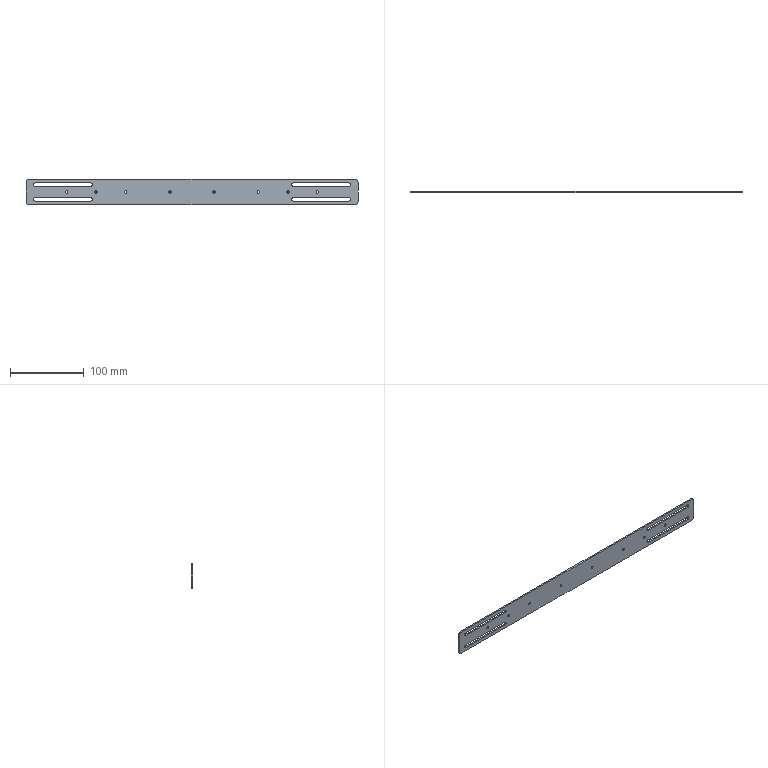Part | SolidWorks | features HoleWzd 3, Fillet 2, Cut 1, EdgeFlange 1, FlatPattern 1, SMBaseFlange 1, SheetMetal 1 | 1 solid | 42 faces | box 450 x 2 x 35 mm | volume 28475 mm3 | cylinder 28 | plane 14 | commonest cylinder face diameters 3.3 x16 4.5 x8 10 x4
STEP:
#1=CARTESIAN_POINT('',(-30.,-2.,-1.65));
#2=VERTEX_POINT('',#1);
#3=CARTESIAN_POINT('',(-30.,-2.,1.65));
#4=VERTEX_POINT('',#3);
#5=CARTESIAN_POINT('',(-30.,-2.,0.));
#6=DIRECTION('',(0.,1.,0.));
#7=DIRECTION('',(0.,0.,1.));
#8=AXIS2_PLACEMENT_3D('',#5,#6,#7);
#9=CIRCLE('',#8,1.65);
#10=EDGE_CURVE('',#2,#4,#9,.T.);
#11=ORIENTED_EDGE('',*,*,#10,.F.);
#12=CARTESIAN_POINT('',(-30.,0.,-1.65));
#13=VERTEX_POINT('',#12);
#14=CARTESIAN_POINT('',(-30.,0.,-1.65));
#15=DIRECTION('',(0.,1.,0.));
#16=VECTOR('',#15,1000.);
#17=LINE('',#14,#16);
#18=EDGE_CURVE('',#2,#13,#17,.T.);
#19=ORIENTED_EDGE('',*,*,#18,.T.);
#20=CARTESIAN_POINT('',(-30.,0.,1.65));
#21=VERTEX_POINT('',#20);
#22=CARTESIAN_POINT('',(-30.,0.,0.));
#23=DIRECTION('',(0.,1.,0.));
#24=DIRECTION('',(0.,0.,1.));
#25=AXIS2_PLACEMENT_3D('',#22,#23,#24);
#26=CIRCLE('',#25,1.65);
#27=EDGE_CURVE('',#13,#21,#26,.T.);
#28=ORIENTED_EDGE('',*,*,#27,.T.);
#29=CARTESIAN_POINT('',(-30.,0.,1.65));
#30=DIRECTION('',(0.,1.,0.));
#31=VECTOR('',#30,1000.);
#32=LINE('',#29,#31);
#33=EDGE_CURVE('',#4,#21,#32,.T.);
#34=ORIENTED_EDGE('',*,*,#33,.F.);
#35=EDGE_LOOP('',(#11,#19,#28,#34));
#36=FACE_OUTER_BOUND('',#35,.T.);
#37=CARTESIAN_POINT('',(-30.,0.,0.));
#38=DIRECTION('',(0.,1.,0.));
#39=DIRECTION('',(0.,0.,1.));
#40=AXIS2_PLACEMENT_3D('',#37,#38,#39);
#41=CYLINDRICAL_SURFACE('',#40,1.65);
#42=ADVANCED_FACE('',(#36),#41,.F.);
#43=CARTESIAN_POINT('',(30.,-2.,-1.65));
#44=VERTEX_POINT('',#43);
#45=CARTESIAN_POINT('',(30.,-2.,1.65));
#46=VERTEX_POINT('',#45);
#47=CARTESIAN_POINT('',(30.,-2.,0.));
#48=DIRECTION('',(0.,1.,0.));
#49=DIRECTION('',(0.,0.,1.));
#50=AXIS2_PLACEMENT_3D('',#47,#48,#49);
#51=CIRCLE('',#50,1.65);
#52=EDGE_CURVE('',#44,#46,#51,.T.);
#53=ORIENTED_EDGE('',*,*,#52,.F.);
#54=CARTESIAN_POINT('',(30.,0.,-1.65));
#55=VERTEX_POINT('',#54);
#56=CARTESIAN_POINT('',(30.,0.,-1.65));
#57=DIRECTION('',(0.,1.,0.));
#58=VECTOR('',#57,1000.);
#59=LINE('',#56,#58);
#60=EDGE_CURVE('',#44,#55,#59,.T.);
#61=ORIENTED_EDGE('',*,*,#60,.T.);
#62=CARTESIAN_POINT('',(30.,0.,1.65));
#63=VERTEX_POINT('',#62);
#64=CARTESIAN_POINT('',(30.,0.,0.));
#65=DIRECTION('',(0.,1.,0.));
#66=DIRECTION('',(0.,0.,1.));
#67=AXIS2_PLACEMENT_3D('',#64,#65,#66);
#68=CIRCLE('',#67,1.65);
#69=EDGE_CURVE('',#55,#63,#68,.T.);
#70=ORIENTED_EDGE('',*,*,#69,.T.);
#71=CARTESIAN_POINT('',(30.,0.,1.65));
#72=DIRECTION('',(0.,1.,0.));
#73=VECTOR('',#72,1000.);
#74=LINE('',#71,#73);
#75=EDGE_CURVE('',#46,#63,#74,.T.);
#76=ORIENTED_EDGE('',*,*,#75,.F.);
#77=EDGE_LOOP('',(#53,#61,#70,#76));
#78=FACE_OUTER_BOUND('',#77,.T.);
#79=CARTESIAN_POINT('',(30.,0.,0.));
#80=DIRECTION('',(0.,1.,0.));
#81=DIRECTION('',(0.,0.,1.));
#82=AXIS2_PLACEMENT_3D('',#79,#80,#81);
#83=CYLINDRICAL_SURFACE('',#82,1.65);
#84=ADVANCED_FACE('',(#78),#83,.F.);
#85=CARTESIAN_POINT('',(-90.,-2.,-1.65));
#86=VERTEX_POINT('',#85);
#87=CARTESIAN_POINT('',(-90.,-2.,1.65));
#88=VERTEX_POINT('',#87);
#89=CARTESIAN_POINT('',(-90.,-2.,0.));
#90=DIRECTION('',(0.,1.,0.));
#91=DIRECTION('',(0.,0.,1.));
#92=AXIS2_PLACEMENT_3D('',#89,#90,#91);
#93=CIRCLE('',#92,1.65);
#94=EDGE_CURVE('',#86,#88,#93,.T.);
#95=ORIENTED_EDGE('',*,*,#94,.F.);
#96=CARTESIAN_POINT('',(-90.,0.,-1.65));
#97=VERTEX_POINT('',#96);
#98=CARTESIAN_POINT('',(-90.,0.,-1.65));
#99=DIRECTION('',(0.,1.,0.));
#100=VECTOR('',#99,1000.);
#101=LINE('',#98,#100);
#102=EDGE_CURVE('',#86,#97,#101,.T.);
#103=ORIENTED_EDGE('',*,*,#102,.T.);
#104=CARTESIAN_POINT('',(-90.,0.,1.65));
#105=VERTEX_POINT('',#104);
#106=CARTESIAN_POINT('',(-90.,0.,0.));
#107=DIRECTION('',(0.,1.,0.));
#108=DIRECTION('',(0.,0.,1.));
#109=AXIS2_PLACEMENT_3D('',#106,#107,#108);
#110=CIRCLE('',#109,1.65);
#111=EDGE_CURVE('',#97,#105,#110,.T.);
#112=ORIENTED_EDGE('',*,*,#111,.T.);
#113=CARTESIAN_POINT('',(-90.,0.,1.65));
#114=DIRECTION('',(0.,1.,0.));
#115=VECTOR('',#114,1000.);
#116=LINE('',#113,#115);
#117=EDGE_CURVE('',#88,#105,#116,.T.);
#118=ORIENTED_EDGE('',*,*,#117,.F.);
#119=EDGE_LOOP('',(#95,#103,#112,#118));
#120=FACE_OUTER_BOUND('',#119,.T.);
#121=CARTESIAN_POINT('',(-90.,0.,0.));
#122=DIRECTION('',(0.,1.,0.));
#123=DIRECTION('',(0.,0.,1.));
#124=AXIS2_PLACEMENT_3D('',#121,#122,#123);
#125=CYLINDRICAL_SURFACE('',#124,1.65);
#126=ADVANCED_FACE('',(#120),#125,.F.);
#127=CARTESIAN_POINT('',(90.,-2.,-1.65));
#128=VERTEX_POINT('',#127);
#129=CARTESIAN_POINT('',(90.,-2.,1.65));
#130=VERTEX_POINT('',#129);
#131=CARTESIAN_POINT('',(90.,-2.,0.));
#132=DIRECTION('',(0.,1.,0.));
#133=DIRECTION('',(0.,0.,1.));
#134=AXIS2_PLACEMENT_3D('',#131,#132,#133);
#135=CIRCLE('',#134,1.65);
#136=EDGE_CURVE('',#128,#130,#135,.T.);
#137=ORIENTED_EDGE('',*,*,#136,.F.);
#138=CARTESIAN_POINT('',(90.,0.,-1.65));
#139=VERTEX_POINT('',#138);
#140=CARTESIAN_POINT('',(90.,0.,-1.65));
#141=DIRECTION('',(0.,1.,0.));
#142=VECTOR('',#141,1000.);
#143=LINE('',#140,#142);
#144=EDGE_CURVE('',#128,#139,#143,.T.);
#145=ORIENTED_EDGE('',*,*,#144,.T.);
#146=CARTESIAN_POINT('',(90.,0.,1.65));
#147=VERTEX_POINT('',#146);
#148=CARTESIAN_POINT('',(90.,0.,0.));
#149=DIRECTION('',(0.,1.,0.));
#150=DIRECTION('',(0.,0.,1.));
#151=AXIS2_PLACEMENT_3D('',#148,#149,#150);
#152=CIRCLE('',#151,1.65);
#153=EDGE_CURVE('',#139,#147,#152,.T.);
#154=ORIENTED_EDGE('',*,*,#153,.T.);
#155=CARTESIAN_POINT('',(90.,0.,1.65));
#156=DIRECTION('',(0.,1.,0.));
#157=VECTOR('',#156,1000.);
#158=LINE('',#155,#157);
#159=EDGE_CURVE('',#130,#147,#158,.T.);
#160=ORIENTED_EDGE('',*,*,#159,.F.);
#161=EDGE_LOOP('',(#137,#145,#154,#160));
#162=FACE_OUTER_BOUND('',#161,.T.);
#163=CARTESIAN_POINT('',(90.,0.,0.));
#164=DIRECTION('',(0.,1.,0.));
#165=DIRECTION('',(0.,0.,1.));
#166=AXIS2_PLACEMENT_3D('',#163,#164,#165);
#167=CYLINDRICAL_SURFACE('',#166,1.65);
#168=ADVANCED_FACE('',(#162),#167,.F.);
#169=CARTESIAN_POINT('',(-130.,-2.,-1.65));
#170=VERTEX_POINT('',#169);
#171=CARTESIAN_POINT('',(-130.,-2.,1.65));
#172=VERTEX_POINT('',#171);
#173=CARTESIAN_POINT('',(-130.,-2.,0.));
#174=DIRECTION('',(0.,1.,0.));
#175=DIRECTION('',(0.,0.,1.));
#176=AXIS2_PLACEMENT_3D('',#173,#174,#175);
#177=CIRCLE('',#176,1.65);
#178=EDGE_CURVE('',#170,#172,#177,.T.);
#179=ORIENTED_EDGE('',*,*,#178,.F.);
#180=CARTESIAN_POINT('',(-130.,0.,-1.65));
#181=VERTEX_POINT('',#180);
#182=CARTESIAN_POINT('',(-130.,0.,-1.65));
#183=DIRECTION('',(0.,1.,0.));
#184=VECTOR('',#183,1000.);
#185=LINE('',#182,#184);
#186=EDGE_CURVE('',#170,#181,#185,.T.);
#187=ORIENTED_EDGE('',*,*,#186,.T.);
#188=CARTESIAN_POINT('',(-130.,0.,1.65));
#189=VERTEX_POINT('',#188);
#190=CARTESIAN_POINT('',(-130.,0.,0.));
#191=DIRECTION('',(0.,1.,0.));
#192=DIRECTION('',(0.,0.,1.));
#193=AXIS2_PLACEMENT_3D('',#190,#191,#192);
#194=CIRCLE('',#193,1.65);
#195=EDGE_CURVE('',#181,#189,#194,.T.);
#196=ORIENTED_EDGE('',*,*,#195,.T.);
#197=CARTESIAN_POINT('',(-130.,0.,1.65));
#198=DIRECTION('',(0.,1.,0.));
#199=VECTOR('',#198,1000.);
#200=LINE('',#197,#199);
#201=EDGE_CURVE('',#172,#189,#200,.T.);
#202=ORIENTED_EDGE('',*,*,#201,.F.);
#203=EDGE_LOOP('',(#179,#187,#196,#202));
#204=FACE_OUTER_BOUND('',#203,.T.);
#205=CARTESIAN_POINT('',(-130.,0.,0.));
#206=DIRECTION('',(0.,1.,0.));
#207=DIRECTION('',(0.,0.,1.));
#208=AXIS2_PLACEMENT_3D('',#205,#206,#207);
#209=CYLINDRICAL_SURFACE('',#208,1.65);
#210=ADVANCED_FACE('',(#204),#209,.F.);
#211=CARTESIAN_POINT('',(-170.,-2.,-1.65));
#212=VERTEX_POINT('',#211);
#213=CARTESIAN_POINT('',(-170.,-2.,1.65));
#214=VERTEX_POINT('',#213);
#215=CARTESIAN_POINT('',(-170.,-2.,0.));
#216=DIRECTION('',(0.,1.,0.));
#217=DIRECTION('',(0.,0.,1.));
#218=AXIS2_PLACEMENT_3D('',#215,#216,#217);
#219=CIRCLE('',#218,1.65);
#220=EDGE_CURVE('',#212,#214,#219,.T.);
#221=ORIENTED_EDGE('',*,*,#220,.F.);
#222=CARTESIAN_POINT('',(-170.,0.,-1.65));
#223=VERTEX_POINT('',#222);
#224=CARTESIAN_POINT('',(-170.,0.,-1.65));
#225=DIRECTION('',(0.,1.,0.));
#226=VECTOR('',#225,1000.);
#227=LINE('',#224,#226);
#228=EDGE_CURVE('',#212,#223,#227,.T.);
#229=ORIENTED_EDGE('',*,*,#228,.T.);
#230=CARTESIAN_POINT('',(-170.,0.,1.65));
#231=VERTEX_POINT('',#230);
#232=CARTESIAN_POINT('',(-170.,0.,0.));
#233=DIRECTION('',(0.,1.,0.));
#234=DIRECTION('',(0.,0.,1.));
#235=AXIS2_PLACEMENT_3D('',#232,#233,#234);
#236=CIRCLE('',#235,1.65);
#237=EDGE_CURVE('',#223,#231,#236,.T.);
#238=ORIENTED_EDGE('',*,*,#237,.T.);
#239=CARTESIAN_POINT('',(-170.,0.,1.65));
#240=DIRECTION('',(0.,1.,0.));
#241=VECTOR('',#240,1000.);
#242=LINE('',#239,#241);
#243=EDGE_CURVE('',#214,#231,#242,.T.);
#244=ORIENTED_EDGE('',*,*,#243,.F.);
#245=EDGE_LOOP('',(#221,#229,#238,#244));
#246=FACE_OUTER_BOUND('',#245,.T.);
#247=CARTESIAN_POINT('',(-170.,0.,0.));
#248=DIRECTION('',(0.,1.,0.));
#249=DIRECTION('',(0.,0.,1.));
#250=AXIS2_PLACEMENT_3D('',#247,#248,#249);
#251=CYLINDRICAL_SURFACE('',#250,1.65);
#252=ADVANCED_FACE('',(#246),#251,.F.);
#253=CARTESIAN_POINT('',(130.,-2.,-1.65));
#254=VERTEX_POINT('',#253);
#255=CARTESIAN_POINT('',(130.,-2.,1.65));
#256=VERTEX_POINT('',#255);
#257=CARTESIAN_POINT('',(130.,-2.,0.));
#258=DIRECTION('',(0.,1.,0.));
#259=DIRECTION('',(0.,0.,1.));
#260=AXIS2_PLACEMENT_3D('',#257,#258,#259);
#261=CIRCLE('',#260,1.65);
#262=EDGE_CURVE('',#254,#256,#261,.T.);
#263=ORIENTED_EDGE('',*,*,#262,.F.);
#264=CARTESIAN_POINT('',(130.,0.,-1.65));
#265=VERTEX_POINT('',#264);
#266=CARTESIAN_POINT('',(130.,0.,-1.65));
#267=DIRECTION('',(0.,1.,0.));
#268=VECTOR('',#267,1000.);
#269=LINE('',#266,#268);
#270=EDGE_CURVE('',#254,#265,#269,.T.);
#271=ORIENTED_EDGE('',*,*,#270,.T.);
#272=CARTESIAN_POINT('',(130.,0.,1.65));
#273=VERTEX_POINT('',#272);
#274=CARTESIAN_POINT('',(130.,0.,0.));
#275=DIRECTION('',(0.,1.,0.));
#276=DIRECTION('',(0.,0.,1.));
#277=AXIS2_PLACEMENT_3D('',#274,#275,#276);
#278=CIRCLE('',#277,1.65);
#279=EDGE_CURVE('',#265,#273,#278,.T.);
#280=ORIENTED_EDGE('',*,*,#279,.T.);
#281=CARTESIAN_POINT('',(130.,0.,1.65));
#282=DIRECTION('',(0.,1.,0.));
#283=VECTOR('',#282,1000.);
#284=LINE('',#281,#283);
#285=EDGE_CURVE('',#256,#273,#284,.T.);
#286=ORIENTED_EDGE('',*,*,#285,.F.);
#287=EDGE_LOOP('',(#263,#271,#280,#286));
#288=FACE_OUTER_BOUND('',#287,.T.);
#289=CARTESIAN_POINT('',(130.,0.,0.));
#290=DIRECTION('',(0.,1.,0.));
#291=DIRECTION('',(0.,0.,1.));
#292=AXIS2_PLACEMENT_3D('',#289,#290,#291);
#293=CYLINDRICAL_SURFACE('',#292,1.65);
#294=ADVANCED_FACE('',(#288),#293,.F.);
#295=CARTESIAN_POINT('',(170.,-2.,-1.65));
#296=VERTEX_POINT('',#295);
#297=CARTESIAN_POINT('',(170.,-2.,1.65));
#298=VERTEX_POINT('',#297);
#299=CARTESIAN_POINT('',(170.,-2.,0.));
#300=DIRECTION('',(0.,1.,0.));
#301=DIRECTION('',(0.,0.,1.));
#302=AXIS2_PLACEMENT_3D('',#299,#300,#301);
#303=CIRCLE('',#302,1.65);
#304=EDGE_CURVE('',#296,#298,#303,.T.);
#305=ORIENTED_EDGE('',*,*,#304,.F.);
#306=CARTESIAN_POINT('',(170.,0.,-1.65));
#307=VERTEX_POINT('',#306);
#308=CARTESIAN_POINT('',(170.,0.,-1.65));
#309=DIRECTION('',(0.,1.,0.));
#310=VECTOR('',#309,1000.);
#311=LINE('',#308,#310);
#312=EDGE_CURVE('',#296,#307,#311,.T.);
#313=ORIENTED_EDGE('',*,*,#312,.T.);
#314=CARTESIAN_POINT('',(170.,0.,1.65));
#315=VERTEX_POINT('',#314);
#316=CARTESIAN_POINT('',(170.,0.,0.));
#317=DIRECTION('',(0.,1.,0.));
#318=DIRECTION('',(0.,0.,1.));
#319=AXIS2_PLACEMENT_3D('',#316,#317,#318);
#320=CIRCLE('',#319,1.65);
#321=EDGE_CURVE('',#307,#315,#320,.T.);
#322=ORIENTED_EDGE('',*,*,#321,.T.);
#323=CARTESIAN_POINT('',(170.,0.,1.65));
#324=DIRECTION('',(0.,1.,0.));
#325=VECTOR('',#324,1000.);
#326=LINE('',#323,#325);
#327=EDGE_CURVE('',#298,#315,#326,.T.);
#328=ORIENTED_EDGE('',*,*,#327,.F.);
#329=EDGE_LOOP('',(#305,#313,#322,#328));
#330=FACE_OUTER_BOUND('',#329,.T.);
#331=CARTESIAN_POINT('',(170.,0.,0.));
#332=DIRECTION('',(0.,1.,0.));
#333=DIRECTION('',(0.,0.,1.));
#334=AXIS2_PLACEMENT_3D('',#331,#332,#333);
#335=CYLINDRICAL_SURFACE('',#334,1.65);
#336=ADVANCED_FACE('',(#330),#335,.F.);
#337=CARTESIAN_POINT('',(-137.25,0.,7.75));
#338=VERTEX_POINT('',#337);
#339=CARTESIAN_POINT('',(-137.25,0.,12.25));
#340=VERTEX_POINT('',#339);
#341=CARTESIAN_POINT('',(-137.25,0.,10.));
#342=DIRECTION('',(0.,-1.,0.));
#343=DIRECTION('',(0.,0.,-1.));
#344=AXIS2_PLACEMENT_3D('',#341,#342,#343);
#345=CIRCLE('',#344,2.25);
#346=EDGE_CURVE('',#338,#340,#345,.T.);
#347=ORIENTED_EDGE('',*,*,#346,.T.);
#348=CARTESIAN_POINT('',(-212.75,0.,12.25));
#349=VERTEX_POINT('',#348);
#350=CARTESIAN_POINT('',(-212.75,0.,12.25));
#351=DIRECTION('',(1.,0.,0.));
#352=VECTOR('',#351,1000.);
#353=LINE('',#350,#352);
#354=EDGE_CURVE('',#349,#340,#353,.T.);
#355=ORIENTED_EDGE('',*,*,#354,.F.);
#356=CARTESIAN_POINT('',(-212.75,0.,7.75));
#357=VERTEX_POINT('',#356);
#358=CARTESIAN_POINT('',(-212.75,0.,10.));
#359=DIRECTION('',(0.,-1.,0.));
#360=DIRECTION('',(0.,0.,-1.));
#361=AXIS2_PLACEMENT_3D('',#358,#359,#360);
#362=CIRCLE('',#361,2.25);
#363=EDGE_CURVE('',#349,#357,#362,.T.);
#364=ORIENTED_EDGE('',*,*,#363,.T.);
#365=CARTESIAN_POINT('',(-212.75,0.,7.75));
#366=DIRECTION('',(1.,0.,0.));
#367=VECTOR('',#366,1000.);
#368=LINE('',#365,#367);
#369=EDGE_CURVE('',#357,#338,#368,.T.);
#370=ORIENTED_EDGE('',*,*,#369,.T.);
#371=EDGE_LOOP('',(#347,#355,#364,#370));
#372=FACE_BOUND('',#371,.T.);
#373=CARTESIAN_POINT('',(212.75,0.,-12.25));
#374=VERTEX_POINT('',#373);
#375=CARTESIAN_POINT('',(212.75,0.,-7.75));
#376=VERTEX_POINT('',#375);
#377=CARTESIAN_POINT('',(212.75,0.,-10.));
#378=DIRECTION('',(0.,-1.,0.));
#379=DIRECTION('',(0.,0.,-1.));
#380=AXIS2_PLACEMENT_3D('',#377,#378,#379);
#381=CIRCLE('',#380,2.25);
#382=EDGE_CURVE('',#374,#376,#381,.T.);
#383=ORIENTED_EDGE('',*,*,#382,.T.);
#384=CARTESIAN_POINT('',(137.25,0.,-7.75));
#385=VERTEX_POINT('',#384);
#386=CARTESIAN_POINT('',(137.25,0.,-7.75));
#387=DIRECTION('',(1.,0.,0.));
#388=VECTOR('',#387,1000.);
#389=LINE('',#386,#388);
#390=EDGE_CURVE('',#385,#376,#389,.T.);
#391=ORIENTED_EDGE('',*,*,#390,.F.);
#392=CARTESIAN_POINT('',(137.25,0.,-12.25));
#393=VERTEX_POINT('',#392);
#394=CARTESIAN_POINT('',(137.25,0.,-10.));
#395=DIRECTION('',(0.,-1.,0.));
#396=DIRECTION('',(0.,0.,-1.));
#397=AXIS2_PLACEMENT_3D('',#394,#395,#396);
#398=CIRCLE('',#397,2.25);
#399=EDGE_CURVE('',#385,#393,#398,.T.);
#400=ORIENTED_EDGE('',*,*,#399,.T.);
#401=CARTESIAN_POINT('',(137.25,0.,-12.25));
#402=DIRECTION('',(1.,0.,0.));
#403=VECTOR('',#402,1000.);
#404=LINE('',#401,#403);
#405=EDGE_CURVE('',#393,#374,#404,.T.);
#406=ORIENTED_EDGE('',*,*,#405,.T.);
#407=EDGE_LOOP('',(#383,#391,#400,#406));
#408=FACE_BOUND('',#407,.T.);
#409=CARTESIAN_POINT('',(-137.25,0.,-12.25));
#410=VERTEX_POINT('',#409);
#411=CARTESIAN_POINT('',(-137.25,0.,-7.75));
#412=VERTEX_POINT('',#411);
#413=CARTESIAN_POINT('',(-137.25,0.,-10.));
#414=DIRECTION('',(0.,-1.,0.));
#415=DIRECTION('',(0.,0.,-1.));
#416=AXIS2_PLACEMENT_3D('',#413,#414,#415);
#417=CIRCLE('',#416,2.25);
#418=EDGE_CURVE('',#410,#412,#417,.T.);
#419=ORIENTED_EDGE('',*,*,#418,.T.);
#420=CARTESIAN_POINT('',(-212.75,0.,-7.75));
#421=VERTEX_POINT('',#420);
#422=CARTESIAN_POINT('',(-212.75,0.,-7.75));
#423=DIRECTION('',(1.,0.,0.));
#424=VECTOR('',#423,1000.);
#425=LINE('',#422,#424);
#426=EDGE_CURVE('',#421,#412,#425,.T.);
#427=ORIENTED_EDGE('',*,*,#426,.F.);
#428=CARTESIAN_POINT('',(-212.75,0.,-12.25));
#429=VERTEX_POINT('',#428);
#430=CARTESIAN_POINT('',(-212.75,0.,-10.));
#431=DIRECTION('',(0.,-1.,0.));
#432=DIRECTION('',(0.,0.,-1.));
#433=AXIS2_PLACEMENT_3D('',#430,#431,#432);
#434=CIRCLE('',#433,2.25);
#435=EDGE_CURVE('',#421,#429,#434,.T.);
#436=ORIENTED_EDGE('',*,*,#435,.T.);
#437=CARTESIAN_POINT('',(-212.75,0.,-12.25));
#438=DIRECTION('',(1.,0.,0.));
#439=VECTOR('',#438,1000.);
#440=LINE('',#437,#439);
#441=EDGE_CURVE('',#429,#410,#440,.T.);
#442=ORIENTED_EDGE('',*,*,#441,.T.);
#443=EDGE_LOOP('',(#419,#427,#436,#442));
#444=FACE_BOUND('',#443,.T.);
#445=CARTESIAN_POINT('',(-30.,0.,0.));
#446=DIRECTION('',(0.,1.,0.));
#447=DIRECTION('',(0.,0.,1.));
#448=AXIS2_PLACEMENT_3D('',#445,#446,#447);
#449=CIRCLE('',#448,1.65);
#450=EDGE_CURVE('',#21,#13,#449,.T.);
#451=ORIENTED_EDGE('',*,*,#450,.F.);
#452=ORIENTED_EDGE('',*,*,#27,.F.);
#453=EDGE_LOOP('',(#451,#452));
#454=FACE_BOUND('',#453,.T.);
#455=CARTESIAN_POINT('',(30.,0.,0.));
#456=DIRECTION('',(0.,1.,0.));
#457=DIRECTION('',(0.,0.,1.));
#458=AXIS2_PLACEMENT_3D('',#455,#456,#457);
#459=CIRCLE('',#458,1.65);
#460=EDGE_CURVE('',#63,#55,#459,.T.);
#461=ORIENTED_EDGE('',*,*,#460,.F.);
#462=ORIENTED_EDGE('',*,*,#69,.F.);
#463=EDGE_LOOP('',(#461,#462));
#464=FACE_BOUND('',#463,.T.);
#465=CARTESIAN_POINT('',(-90.,0.,0.));
#466=DIRECTION('',(0.,1.,0.));
#467=DIRECTION('',(0.,0.,1.));
#468=AXIS2_PLACEMENT_3D('',#465,#466,#467);
#469=CIRCLE('',#468,1.65);
#470=EDGE_CURVE('',#105,#97,#469,.T.);
#471=ORIENTED_EDGE('',*,*,#470,.F.);
#472=ORIENTED_EDGE('',*,*,#111,.F.);
#473=EDGE_LOOP('',(#471,#472));
#474=FACE_BOUND('',#473,.T.);
#475=CARTESIAN_POINT('',(90.,0.,0.));
#476=DIRECTION('',(0.,1.,0.));
#477=DIRECTION('',(0.,0.,1.));
#478=AXIS2_PLACEMENT_3D('',#475,#476,#477);
#479=CIRCLE('',#478,1.65);
#480=EDGE_CURVE('',#147,#139,#479,.T.);
#481=ORIENTED_EDGE('',*,*,#480,.F.);
#482=ORIENTED_EDGE('',*,*,#153,.F.);
#483=EDGE_LOOP('',(#481,#482));
#484=FACE_BOUND('',#483,.T.);
#485=CARTESIAN_POINT('',(-130.,0.,0.));
#486=DIRECTION('',(0.,1.,0.));
#487=DIRECTION('',(0.,0.,1.));
#488=AXIS2_PLACEMENT_3D('',#485,#486,#487);
#489=CIRCLE('',#488,1.65);
#490=EDGE_CURVE('',#189,#181,#489,.T.);
#491=ORIENTED_EDGE('',*,*,#490,.F.);
#492=ORIENTED_EDGE('',*,*,#195,.F.);
#493=EDGE_LOOP('',(#491,#492));
#494=FACE_BOUND('',#493,.T.);
#495=CARTESIAN_POINT('',(-170.,0.,0.));
#496=DIRECTION('',(0.,1.,0.));
#497=DIRECTION('',(0.,0.,1.));
#498=AXIS2_PLACEMENT_3D('',#495,#496,#497);
#499=CIRCLE('',#498,1.65);
#500=EDGE_CURVE('',#231,#223,#499,.T.);
#501=ORIENTED_EDGE('',*,*,#500,.F.);
#502=ORIENTED_EDGE('',*,*,#237,.F.);
#503=EDGE_LOOP('',(#501,#502));
#504=FACE_BOUND('',#503,.T.);
#505=CARTESIAN_POINT('',(130.,0.,0.));
#506=DIRECTION('',(0.,1.,0.));
#507=DIRECTION('',(0.,0.,1.));
#508=AXIS2_PLACEMENT_3D('',#505,#506,#507);
#509=CIRCLE('',#508,1.65);
#510=EDGE_CURVE('',#273,#265,#509,.T.);
#511=ORIENTED_EDGE('',*,*,#510,.F.);
#512=ORIENTED_EDGE('',*,*,#279,.F.);
#513=EDGE_LOOP('',(#511,#512));
#514=FACE_BOUND('',#513,.T.);
#515=CARTESIAN_POINT('',(170.,0.,0.));
#516=DIRECTION('',(0.,1.,0.));
#517=DIRECTION('',(0.,0.,1.));
#518=AXIS2_PLACEMENT_3D('',#515,#516,#517);
#519=CIRCLE('',#518,1.65);
#520=EDGE_CURVE('',#315,#307,#519,.T.);
#521=ORIENTED_EDGE('',*,*,#520,.F.);
#522=ORIENTED_EDGE('',*,*,#321,.F.);
#523=EDGE_LOOP('',(#521,#522));
#524=FACE_BOUND('',#523,.T.);
#525=CARTESIAN_POINT('',(-220.,0.,17.5));
#526=VERTEX_POINT('',#525);
#527=CARTESIAN_POINT('',(220.,0.,17.5));
#528=VERTEX_POINT('',#527);
#529=CARTESIAN_POINT('',(-225.,0.,17.5));
#530=DIRECTION('',(1.,0.,0.));
#531=VECTOR('',#530,1000.);
#532=LINE('',#529,#531);
#533=EDGE_CURVE('',#526,#528,#532,.T.);
#534=ORIENTED_EDGE('',*,*,#533,.T.);
#535=CARTESIAN_POINT('',(225.,0.,12.5));
#536=VERTEX_POINT('',#535);
#537=CARTESIAN_POINT('',(220.,0.,12.5));
#538=DIRECTION('',(0.,1.,0.));
#539=DIRECTION('',(0.,0.,1.));
#540=AXIS2_PLACEMENT_3D('',#537,#538,#539);
#541=CIRCLE('',#540,5.);
#542=EDGE_CURVE('',#528,#536,#541,.T.);
#543=ORIENTED_EDGE('',*,*,#542,.T.);
#544=CARTESIAN_POINT('',(225.,0.,-12.5));
#545=VERTEX_POINT('',#544);
#546=CARTESIAN_POINT('',(225.,0.,-17.5));
#547=DIRECTION('',(0.,0.,-1.));
#548=VECTOR('',#547,1000.);
#549=LINE('',#546,#548);
#550=EDGE_CURVE('',#536,#545,#549,.T.);
#551=ORIENTED_EDGE('',*,*,#550,.T.);
#552=CARTESIAN_POINT('',(220.,0.,-17.5));
#553=VERTEX_POINT('',#552);
#554=CARTESIAN_POINT('',(220.,0.,-12.5));
#555=DIRECTION('',(0.,1.,0.));
#556=DIRECTION('',(0.,0.,1.));
#557=AXIS2_PLACEMENT_3D('',#554,#555,#556);
#558=CIRCLE('',#557,5.);
#559=EDGE_CURVE('',#545,#553,#558,.T.);
#560=ORIENTED_EDGE('',*,*,#559,.T.);
#561=CARTESIAN_POINT('',(-220.,0.,-17.5));
#562=VERTEX_POINT('',#561);
#563=CARTESIAN_POINT('',(-225.,0.,-17.5));
#564=DIRECTION('',(-1.,0.,0.));
#565=VECTOR('',#564,1000.);
#566=LINE('',#563,#565);
#567=EDGE_CURVE('',#553,#562,#566,.T.);
#568=ORIENTED_EDGE('',*,*,#567,.T.);
#569=CARTESIAN_POINT('',(-225.,0.,-12.5));
#570=VERTEX_POINT('',#569);
#571=CARTESIAN_POINT('',(-220.,0.,-12.5));
#572=DIRECTION('',(0.,1.,0.));
#573=DIRECTION('',(0.,0.,1.));
#574=AXIS2_PLACEMENT_3D('',#571,#572,#573);
#575=CIRCLE('',#574,5.);
#576=EDGE_CURVE('',#562,#570,#575,.T.);
#577=ORIENTED_EDGE('',*,*,#576,.T.);
#578=CARTESIAN_POINT('',(-225.,0.,12.5));
#579=VERTEX_POINT('',#578);
#580=CARTESIAN_POINT('',(-225.,0.,-17.5));
#581=DIRECTION('',(0.,0.,1.));
#582=VECTOR('',#581,1000.);
#583=LINE('',#580,#582);
#584=EDGE_CURVE('',#570,#579,#583,.T.);
#585=ORIENTED_EDGE('',*,*,#584,.T.);
#586=CARTESIAN_POINT('',(-220.,0.,12.5));
#587=DIRECTION('',(0.,1.,0.));
#588=DIRECTION('',(0.,0.,1.));
#589=AXIS2_PLACEMENT_3D('',#586,#587,#588);
#590=CIRCLE('',#589,5.);
#591=EDGE_CURVE('',#579,#526,#590,.T.);
#592=ORIENTED_EDGE('',*,*,#591,.T.);
#593=EDGE_LOOP('',(#534,#543,#551,#560,#568,#577,#585,#592));
#594=FACE_OUTER_BOUND('',#593,.T.);
#595=CARTESIAN_POINT('',(137.25,0.,12.25));
#596=VERTEX_POINT('',#595);
#597=CARTESIAN_POINT('',(212.75,0.,12.25));
#598=VERTEX_POINT('',#597);
#599=CARTESIAN_POINT('',(137.25,0.,12.25));
#600=DIRECTION('',(1.,0.,0.));
#601=VECTOR('',#600,1000.);
#602=LINE('',#599,#601);
#603=EDGE_CURVE('',#596,#598,#602,.T.);
#604=ORIENTED_EDGE('',*,*,#603,.F.);
#605=CARTESIAN_POINT('',(137.25,0.,7.75));
#606=VERTEX_POINT('',#605);
#607=CARTESIAN_POINT('',(137.25,0.,10.));
#608=DIRECTION('',(0.,-1.,0.));
#609=DIRECTION('',(0.,0.,-1.));
#610=AXIS2_PLACEMENT_3D('',#607,#608,#609);
#611=CIRCLE('',#610,2.25);
#612=EDGE_CURVE('',#596,#606,#611,.T.);
#613=ORIENTED_EDGE('',*,*,#612,.T.);
#614=CARTESIAN_POINT('',(212.75,0.,7.75));
#615=VERTEX_POINT('',#614);
#616=CARTESIAN_POINT('',(137.25,0.,7.75));
#617=DIRECTION('',(1.,0.,0.));
#618=VECTOR('',#617,1000.);
#619=LINE('',#616,#618);
#620=EDGE_CURVE('',#606,#615,#619,.T.);
#621=ORIENTED_EDGE('',*,*,#620,.T.);
#622=CARTESIAN_POINT('',(212.75,0.,10.));
#623=DIRECTION('',(0.,-1.,0.));
#624=DIRECTION('',(0.,0.,-1.));
#625=AXIS2_PLACEMENT_3D('',#622,#623,#624);
#626=CIRCLE('',#625,2.25);
#627=EDGE_CURVE('',#615,#598,#626,.T.);
#628=ORIENTED_EDGE('',*,*,#627,.T.);
#629=EDGE_LOOP('',(#604,#613,#621,#628));
#630=FACE_BOUND('',#629,.T.);
#631=CARTESIAN_POINT('',(0.,0.,0.));
#632=DIRECTION('',(0.,1.,0.));
#633=DIRECTION('',(0.,0.,1.));
#634=AXIS2_PLACEMENT_3D('',#631,#632,#633);
#635=PLANE('',#634);
#636=ADVANCED_FACE('',(#372,#408,#444,#454,#464,#474,#484,#494,#504,#514,#524,#594,#630),#635,.T.);
#637=CARTESIAN_POINT('',(-212.75,-2.,12.25));
#638=VERTEX_POINT('',#637);
#639=CARTESIAN_POINT('',(-137.25,-2.,12.25));
#640=VERTEX_POINT('',#639);
#641=CARTESIAN_POINT('',(-212.75,-2.,12.25));
#642=DIRECTION('',(1.,0.,0.));
#643=VECTOR('',#642,1000.);
#644=LINE('',#641,#643);
#645=EDGE_CURVE('',#638,#640,#644,.T.);
#646=ORIENTED_EDGE('',*,*,#645,.T.);
#647=CARTESIAN_POINT('',(-137.25,-2.,7.75));
#648=VERTEX_POINT('',#647);
#649=CARTESIAN_POINT('',(-137.25,-2.,10.));
#650=DIRECTION('',(0.,-1.,0.));
#651=DIRECTION('',(0.,0.,-1.));
#652=AXIS2_PLACEMENT_3D('',#649,#650,#651);
#653=CIRCLE('',#652,2.25);
#654=EDGE_CURVE('',#648,#640,#653,.T.);
#655=ORIENTED_EDGE('',*,*,#654,.F.);
#656=CARTESIAN_POINT('',(-212.75,-2.,7.75));
#657=VERTEX_POINT('',#656);
#658=CARTESIAN_POINT('',(-212.75,-2.,7.75));
#659=DIRECTION('',(1.,0.,0.));
#660=VECTOR('',#659,1000.);
#661=LINE('',#658,#660);
#662=EDGE_CURVE('',#657,#648,#661,.T.);
#663=ORIENTED_EDGE('',*,*,#662,.F.);
#664=CARTESIAN_POINT('',(-212.75,-2.,10.));
#665=DIRECTION('',(0.,-1.,0.));
#666=DIRECTION('',(0.,0.,-1.));
#667=AXIS2_PLACEMENT_3D('',#664,#665,#666);
#668=CIRCLE('',#667,2.25);
#669=EDGE_CURVE('',#638,#657,#668,.T.);
#670=ORIENTED_EDGE('',*,*,#669,.F.);
#671=EDGE_LOOP('',(#646,#655,#663,#670));
#672=FACE_BOUND('',#671,.T.);
#673=CARTESIAN_POINT('',(137.25,-2.,12.25));
#674=VERTEX_POINT('',#673);
#675=CARTESIAN_POINT('',(212.75,-2.,12.25));
#676=VERTEX_POINT('',#675);
#677=CARTESIAN_POINT('',(137.25,-2.,12.25));
#678=DIRECTION('',(1.,0.,0.));
#679=VECTOR('',#678,1000.);
#680=LINE('',#677,#679);
#681=EDGE_CURVE('',#674,#676,#680,.T.);
#682=ORIENTED_EDGE('',*,*,#681,.T.);
#683=CARTESIAN_POINT('',(212.75,-2.,7.75));
#684=VERTEX_POINT('',#683);
#685=CARTESIAN_POINT('',(212.75,-2.,10.));
#686=DIRECTION('',(0.,-1.,0.));
#687=DIRECTION('',(0.,0.,-1.));
#688=AXIS2_PLACEMENT_3D('',#685,#686,#687);
#689=CIRCLE('',#688,2.25);
#690=EDGE_CURVE('',#684,#676,#689,.T.);
#691=ORIENTED_EDGE('',*,*,#690,.F.);
#692=CARTESIAN_POINT('',(137.25,-2.,7.75));
#693=VERTEX_POINT('',#692);
#694=CARTESIAN_POINT('',(137.25,-2.,7.75));
#695=DIRECTION('',(1.,0.,0.));
#696=VECTOR('',#695,1000.);
#697=LINE('',#694,#696);
#698=EDGE_CURVE('',#693,#684,#697,.T.);
#699=ORIENTED_EDGE('',*,*,#698,.F.);
#700=CARTESIAN_POINT('',(137.25,-2.,10.));
#701=DIRECTION('',(0.,-1.,0.));
#702=DIRECTION('',(0.,0.,-1.));
#703=AXIS2_PLACEMENT_3D('',#700,#701,#702);
#704=CIRCLE('',#703,2.25);
#705=EDGE_CURVE('',#674,#693,#704,.T.);
#706=ORIENTED_EDGE('',*,*,#705,.F.);
#707=EDGE_LOOP('',(#682,#691,#699,#706));
#708=FACE_BOUND('',#707,.T.);
#709=CARTESIAN_POINT('',(212.75,-2.,-12.25));
#710=VERTEX_POINT('',#709);
#711=CARTESIAN_POINT('',(212.75,-2.,-7.75));
#712=VERTEX_POINT('',#711);
#713=CARTESIAN_POINT('',(212.75,-2.,-10.));
#714=DIRECTION('',(0.,-1.,0.));
#715=DIRECTION('',(0.,0.,-1.));
#716=AXIS2_PLACEMENT_3D('',#713,#714,#715);
#717=CIRCLE('',#716,2.25);
#718=EDGE_CURVE('',#710,#712,#717,.T.);
#719=ORIENTED_EDGE('',*,*,#718,.F.);
#720=CARTESIAN_POINT('',(137.25,-2.,-12.25));
#721=VERTEX_POINT('',#720);
#722=CARTESIAN_POINT('',(137.25,-2.,-12.25));
#723=DIRECTION('',(1.,0.,0.));
#724=VECTOR('',#723,1000.);
#725=LINE('',#722,#724);
#726=EDGE_CURVE('',#721,#710,#725,.T.);
#727=ORIENTED_EDGE('',*,*,#726,.F.);
#728=CARTESIAN_POINT('',(137.25,-2.,-7.75));
#729=VERTEX_POINT('',#728);
#730=CARTESIAN_POINT('',(137.25,-2.,-10.));
#731=DIRECTION('',(0.,-1.,0.));
#732=DIRECTION('',(0.,0.,-1.));
#733=AXIS2_PLACEMENT_3D('',#730,#731,#732);
#734=CIRCLE('',#733,2.25);
#735=EDGE_CURVE('',#729,#721,#734,.T.);
#736=ORIENTED_EDGE('',*,*,#735,.F.);
#737=CARTESIAN_POINT('',(137.25,-2.,-7.75));
#738=DIRECTION('',(1.,0.,0.));
#739=VECTOR('',#738,1000.);
#740=LINE('',#737,#739);
#741=EDGE_CURVE('',#729,#712,#740,.T.);
#742=ORIENTED_EDGE('',*,*,#741,.T.);
#743=EDGE_LOOP('',(#719,#727,#736,#742));
#744=FACE_BOUND('',#743,.T.);
#745=CARTESIAN_POINT('',(225.,-2.,12.5));
#746=VERTEX_POINT('',#745);
#747=CARTESIAN_POINT('',(225.,-2.,-12.5));
#748=VERTEX_POINT('',#747);
#749=CARTESIAN_POINT('',(225.,-2.,-17.5));
#750=DIRECTION('',(0.,0.,-1.));
#751=VECTOR('',#750,1000.);
#752=LINE('',#749,#751);
#753=EDGE_CURVE('',#746,#748,#752,.T.);
#754=ORIENTED_EDGE('',*,*,#753,.F.);
#755=CARTESIAN_POINT('',(220.,-2.,17.5));
#756=VERTEX_POINT('',#755);
#757=CARTESIAN_POINT('',(220.,-2.,12.5));
#758=DIRECTION('',(0.,-1.,0.));
#759=DIRECTION('',(0.,0.,1.));
#760=AXIS2_PLACEMENT_3D('',#757,#758,#759);
#761=CIRCLE('',#760,5.);
#762=EDGE_CURVE('',#746,#756,#761,.T.);
#763=ORIENTED_EDGE('',*,*,#762,.T.);
#764=CARTESIAN_POINT('',(-220.,-2.,17.5));
#765=VERTEX_POINT('',#764);
#766=CARTESIAN_POINT('',(-225.,-2.,17.5));
#767=DIRECTION('',(1.,0.,0.));
#768=VECTOR('',#767,1000.);
#769=LINE('',#766,#768);
#770=EDGE_CURVE('',#765,#756,#769,.T.);
#771=ORIENTED_EDGE('',*,*,#770,.F.);
#772=CARTESIAN_POINT('',(-225.,-2.,12.5));
#773=VERTEX_POINT('',#772);
#774=CARTESIAN_POINT('',(-220.,-2.,12.5));
#775=DIRECTION('',(0.,-1.,0.));
#776=DIRECTION('',(0.,0.,1.));
#777=AXIS2_PLACEMENT_3D('',#774,#775,#776);
#778=CIRCLE('',#777,5.);
#779=EDGE_CURVE('',#765,#773,#778,.T.);
#780=ORIENTED_EDGE('',*,*,#779,.T.);
#781=CARTESIAN_POINT('',(-225.,-2.,-12.5));
#782=VERTEX_POINT('',#781);
#783=CARTESIAN_POINT('',(-225.,-2.,-17.5));
#784=DIRECTION('',(0.,0.,1.));
#785=VECTOR('',#784,1000.);
#786=LINE('',#783,#785);
#787=EDGE_CURVE('',#782,#773,#786,.T.);
#788=ORIENTED_EDGE('',*,*,#787,.F.);
#789=CARTESIAN_POINT('',(-220.,-2.,-17.5));
#790=VERTEX_POINT('',#789);
#791=CARTESIAN_POINT('',(-220.,-2.,-12.5));
#792=DIRECTION('',(0.,-1.,0.));
#793=DIRECTION('',(0.,0.,1.));
#794=AXIS2_PLACEMENT_3D('',#791,#792,#793);
#795=CIRCLE('',#794,5.);
#796=EDGE_CURVE('',#782,#790,#795,.T.);
#797=ORIENTED_EDGE('',*,*,#796,.T.);
#798=CARTESIAN_POINT('',(220.,-2.,-17.5));
#799=VERTEX_POINT('',#798);
#800=CARTESIAN_POINT('',(-225.,-2.,-17.5));
#801=DIRECTION('',(-1.,0.,0.));
#802=VECTOR('',#801,1000.);
#803=LINE('',#800,#802);
#804=EDGE_CURVE('',#799,#790,#803,.T.);
#805=ORIENTED_EDGE('',*,*,#804,.F.);
#806=CARTESIAN_POINT('',(220.,-2.,-12.5));
#807=DIRECTION('',(0.,-1.,0.));
#808=DIRECTION('',(0.,0.,1.));
#809=AXIS2_PLACEMENT_3D('',#806,#807,#808);
#810=CIRCLE('',#809,5.);
#811=EDGE_CURVE('',#799,#748,#810,.T.);
#812=ORIENTED_EDGE('',*,*,#811,.T.);
#813=EDGE_LOOP('',(#754,#763,#771,#780,#788,#797,#805,#812));
#814=FACE_OUTER_BOUND('',#813,.T.);
#815=CARTESIAN_POINT('',(170.,-2.,0.));
#816=DIRECTION('',(0.,1.,0.));
#817=DIRECTION('',(0.,0.,1.));
#818=AXIS2_PLACEMENT_3D('',#815,#816,#817);
#819=CIRCLE('',#818,1.65);
#820=EDGE_CURVE('',#298,#296,#819,.T.);
#821=ORIENTED_EDGE('',*,*,#820,.T.);
#822=ORIENTED_EDGE('',*,*,#304,.T.);
#823=EDGE_LOOP('',(#821,#822));
#824=FACE_BOUND('',#823,.T.);
#825=CARTESIAN_POINT('',(130.,-2.,0.));
#826=DIRECTION('',(0.,1.,0.));
#827=DIRECTION('',(0.,0.,1.));
#828=AXIS2_PLACEMENT_3D('',#825,#826,#827);
#829=CIRCLE('',#828,1.65);
#830=EDGE_CURVE('',#256,#254,#829,.T.);
#831=ORIENTED_EDGE('',*,*,#830,.T.);
#832=ORIENTED_EDGE('',*,*,#262,.T.);
#833=EDGE_LOOP('',(#831,#832));
#834=FACE_BOUND('',#833,.T.);
#835=CARTESIAN_POINT('',(-170.,-2.,0.));
#836=DIRECTION('',(0.,1.,0.));
#837=DIRECTION('',(0.,0.,1.));
#838=AXIS2_PLACEMENT_3D('',#835,#836,#837);
#839=CIRCLE('',#838,1.65);
#840=EDGE_CURVE('',#214,#212,#839,.T.);
#841=ORIENTED_EDGE('',*,*,#840,.T.);
#842=ORIENTED_EDGE('',*,*,#220,.T.);
#843=EDGE_LOOP('',(#841,#842));
#844=FACE_BOUND('',#843,.T.);
#845=CARTESIAN_POINT('',(-130.,-2.,0.));
#846=DIRECTION('',(0.,1.,0.));
#847=DIRECTION('',(0.,0.,1.));
#848=AXIS2_PLACEMENT_3D('',#845,#846,#847);
#849=CIRCLE('',#848,1.65);
#850=EDGE_CURVE('',#172,#170,#849,.T.);
#851=ORIENTED_EDGE('',*,*,#850,.T.);
#852=ORIENTED_EDGE('',*,*,#178,.T.);
#853=EDGE_LOOP('',(#851,#852));
#854=FACE_BOUND('',#853,.T.);
#855=CARTESIAN_POINT('',(90.,-2.,0.));
#856=DIRECTION('',(0.,1.,0.));
#857=DIRECTION('',(0.,0.,1.));
#858=AXIS2_PLACEMENT_3D('',#855,#856,#857);
#859=CIRCLE('',#858,1.65);
#860=EDGE_CURVE('',#130,#128,#859,.T.);
#861=ORIENTED_EDGE('',*,*,#860,.T.);
#862=ORIENTED_EDGE('',*,*,#136,.T.);
#863=EDGE_LOOP('',(#861,#862));
#864=FACE_BOUND('',#863,.T.);
#865=CARTESIAN_POINT('',(-90.,-2.,0.));
#866=DIRECTION('',(0.,1.,0.));
#867=DIRECTION('',(0.,0.,1.));
#868=AXIS2_PLACEMENT_3D('',#865,#866,#867);
#869=CIRCLE('',#868,1.65);
#870=EDGE_CURVE('',#88,#86,#869,.T.);
#871=ORIENTED_EDGE('',*,*,#870,.T.);
#872=ORIENTED_EDGE('',*,*,#94,.T.);
#873=EDGE_LOOP('',(#871,#872));
#874=FACE_BOUND('',#873,.T.);
#875=CARTESIAN_POINT('',(30.,-2.,0.));
#876=DIRECTION('',(0.,1.,0.));
#877=DIRECTION('',(0.,0.,1.));
#878=AXIS2_PLACEMENT_3D('',#875,#876,#877);
#879=CIRCLE('',#878,1.65);
#880=EDGE_CURVE('',#46,#44,#879,.T.);
#881=ORIENTED_EDGE('',*,*,#880,.T.);
#882=ORIENTED_EDGE('',*,*,#52,.T.);
#883=EDGE_LOOP('',(#881,#882));
#884=FACE_BOUND('',#883,.T.);
#885=CARTESIAN_POINT('',(-30.,-2.,0.));
#886=DIRECTION('',(0.,1.,0.));
#887=DIRECTION('',(0.,0.,1.));
#888=AXIS2_PLACEMENT_3D('',#885,#886,#887);
#889=CIRCLE('',#888,1.65);
#890=EDGE_CURVE('',#4,#2,#889,.T.);
#891=ORIENTED_EDGE('',*,*,#890,.T.);
#892=ORIENTED_EDGE('',*,*,#10,.T.);
#893=EDGE_LOOP('',(#891,#892));
#894=FACE_BOUND('',#893,.T.);
#895=CARTESIAN_POINT('',(-212.75,-2.,-12.25));
#896=VERTEX_POINT('',#895);
#897=CARTESIAN_POINT('',(-137.25,-2.,-12.25));
#898=VERTEX_POINT('',#897);
#899=CARTESIAN_POINT('',(-212.75,-2.,-12.25));
#900=DIRECTION('',(1.,0.,0.));
#901=VECTOR('',#900,1000.);
#902=LINE('',#899,#901);
#903=EDGE_CURVE('',#896,#898,#902,.T.);
#904=ORIENTED_EDGE('',*,*,#903,.F.);
#905=CARTESIAN_POINT('',(-212.75,-2.,-7.75));
#906=VERTEX_POINT('',#905);
#907=CARTESIAN_POINT('',(-212.75,-2.,-10.));
#908=DIRECTION('',(0.,-1.,0.));
#909=DIRECTION('',(0.,0.,-1.));
#910=AXIS2_PLACEMENT_3D('',#907,#908,#909);
#911=CIRCLE('',#910,2.25);
#912=EDGE_CURVE('',#906,#896,#911,.T.);
#913=ORIENTED_EDGE('',*,*,#912,.F.);
#914=CARTESIAN_POINT('',(-137.25,-2.,-7.75));
#915=VERTEX_POINT('',#914);
#916=CARTESIAN_POINT('',(-212.75,-2.,-7.75));
#917=DIRECTION('',(1.,0.,0.));
#918=VECTOR('',#917,1000.);
#919=LINE('',#916,#918);
#920=EDGE_CURVE('',#906,#915,#919,.T.);
#921=ORIENTED_EDGE('',*,*,#920,.T.);
#922=CARTESIAN_POINT('',(-137.25,-2.,-10.));
#923=DIRECTION('',(0.,-1.,0.));
#924=DIRECTION('',(0.,0.,-1.));
#925=AXIS2_PLACEMENT_3D('',#922,#923,#924);
#926=CIRCLE('',#925,2.25);
#927=EDGE_CURVE('',#898,#915,#926,.T.);
#928=ORIENTED_EDGE('',*,*,#927,.F.);
#929=EDGE_LOOP('',(#904,#913,#921,#928));
#930=FACE_BOUND('',#929,.T.);
#931=CARTESIAN_POINT('',(0.,-2.,0.));
#932=DIRECTION('',(0.,1.,0.));
#933=DIRECTION('',(0.,0.,1.));
#934=AXIS2_PLACEMENT_3D('',#931,#932,#933);
#935=PLANE('',#934);
#936=ADVANCED_FACE('',(#672,#708,#744,#814,#824,#834,#844,#854,#864,#874,#884,#894,#930),#935,.F.);
#937=ORIENTED_EDGE('',*,*,#550,.F.);
#938=CARTESIAN_POINT('',(225.,-2.,12.5));
#939=DIRECTION('',(0.,-1.,0.));
#940=VECTOR('',#939,1000.);
#941=LINE('',#938,#940);
#942=EDGE_CURVE('',#536,#746,#941,.T.);
#943=ORIENTED_EDGE('',*,*,#942,.T.);
#944=ORIENTED_EDGE('',*,*,#753,.T.);
#945=CARTESIAN_POINT('',(225.,-2.,-12.5));
#946=DIRECTION('',(0.,1.,0.));
#947=VECTOR('',#946,1000.);
#948=LINE('',#945,#947);
#949=EDGE_CURVE('',#748,#545,#948,.T.);
#950=ORIENTED_EDGE('',*,*,#949,.T.);
#951=EDGE_LOOP('',(#937,#943,#944,#950));
#952=FACE_OUTER_BOUND('',#951,.T.);
#953=CARTESIAN_POINT('',(225.,-2.,-17.5));
#954=DIRECTION('',(1.,0.,0.));
#955=DIRECTION('',(0.,0.,-1.));
#956=AXIS2_PLACEMENT_3D('',#953,#954,#955);
#957=PLANE('',#956);
#958=ADVANCED_FACE('',(#952),#957,.T.);
#959=ORIENTED_EDGE('',*,*,#770,.T.);
#960=CARTESIAN_POINT('',(220.,-2.,17.5));
#961=DIRECTION('',(0.,1.,0.));
#962=VECTOR('',#961,1000.);
#963=LINE('',#960,#962);
#964=EDGE_CURVE('',#756,#528,#963,.T.);
#965=ORIENTED_EDGE('',*,*,#964,.T.);
#966=ORIENTED_EDGE('',*,*,#533,.F.);
#967=CARTESIAN_POINT('',(-220.,-2.,17.5));
#968=DIRECTION('',(0.,-1.,0.));
#969=VECTOR('',#968,1000.);
#970=LINE('',#967,#969);
#971=EDGE_CURVE('',#526,#765,#970,.T.);
#972=ORIENTED_EDGE('',*,*,#971,.T.);
#973=EDGE_LOOP('',(#959,#965,#966,#972));
#974=FACE_OUTER_BOUND('',#973,.T.);
#975=CARTESIAN_POINT('',(-225.,-2.,17.5));
#976=DIRECTION('',(0.,0.,1.));
#977=DIRECTION('',(1.,0.,0.));
#978=AXIS2_PLACEMENT_3D('',#975,#976,#977);
#979=PLANE('',#978);
#980=ADVANCED_FACE('',(#974),#979,.T.);
#981=ORIENTED_EDGE('',*,*,#787,.T.);
#982=CARTESIAN_POINT('',(-225.,-2.,12.5));
#983=DIRECTION('',(0.,1.,0.));
#984=VECTOR('',#983,1000.);
#985=LINE('',#982,#984);
#986=EDGE_CURVE('',#773,#579,#985,.T.);
#987=ORIENTED_EDGE('',*,*,#986,.T.);
#988=ORIENTED_EDGE('',*,*,#584,.F.);
#989=CARTESIAN_POINT('',(-225.,-2.,-12.5));
#990=DIRECTION('',(0.,-1.,0.));
#991=VECTOR('',#990,1000.);
#992=LINE('',#989,#991);
#993=EDGE_CURVE('',#570,#782,#992,.T.);
#994=ORIENTED_EDGE('',*,*,#993,.T.);
#995=EDGE_LOOP('',(#981,#987,#988,#994));
#996=FACE_OUTER_BOUND('',#995,.T.);
#997=CARTESIAN_POINT('',(-225.,-2.,-17.5));
#998=DIRECTION('',(-1.,0.,0.));
#999=DIRECTION('',(0.,0.,1.));
#1000=AXIS2_PLACEMENT_3D('',#997,#998,#999);
#1001=PLANE('',#1000);
#1002=ADVANCED_FACE('',(#996),#1001,.T.);
#1003=ORIENTED_EDGE('',*,*,#567,.F.);
#1004=CARTESIAN_POINT('',(220.,-2.,-17.5));
#1005=DIRECTION('',(0.,-1.,0.));
#1006=VECTOR('',#1005,1000.);
#1007=LINE('',#1004,#1006);
#1008=EDGE_CURVE('',#553,#799,#1007,.T.);
#1009=ORIENTED_EDGE('',*,*,#1008,.T.);
#1010=ORIENTED_EDGE('',*,*,#804,.T.);
#1011=CARTESIAN_POINT('',(-220.,-2.,-17.5));
#1012=DIRECTION('',(0.,1.,0.));
#1013=VECTOR('',#1012,1000.);
#1014=LINE('',#1011,#1013);
#1015=EDGE_CURVE('',#790,#562,#1014,.T.);
#1016=ORIENTED_EDGE('',*,*,#1015,.T.);
#1017=EDGE_LOOP('',(#1003,#1009,#1010,#1016));
#1018=FACE_OUTER_BOUND('',#1017,.T.);
#1019=CARTESIAN_POINT('',(-225.,-2.,-17.5));
#1020=DIRECTION('',(0.,0.,-1.));
#1021=DIRECTION('',(-1.,0.,0.));
#1022=AXIS2_PLACEMENT_3D('',#1019,#1020,#1021);
#1023=PLANE('',#1022);
#1024=ADVANCED_FACE('',(#1018),#1023,.T.);
#1025=ORIENTED_EDGE('',*,*,#312,.F.);
#1026=ORIENTED_EDGE('',*,*,#820,.F.);
#1027=ORIENTED_EDGE('',*,*,#327,.T.);
#1028=ORIENTED_EDGE('',*,*,#520,.T.);
#1029=EDGE_LOOP('',(#1025,#1026,#1027,#1028));
#1030=FACE_OUTER_BOUND('',#1029,.T.);
#1031=CARTESIAN_POINT('',(170.,0.,0.));
#1032=DIRECTION('',(0.,1.,0.));
#1033=DIRECTION('',(0.,0.,1.));
#1034=AXIS2_PLACEMENT_3D('',#1031,#1032,#1033);
#1035=CYLINDRICAL_SURFACE('',#1034,1.65);
#1036=ADVANCED_FACE('',(#1030),#1035,.F.);
#1037=ORIENTED_EDGE('',*,*,#270,.F.);
#1038=ORIENTED_EDGE('',*,*,#830,.F.);
#1039=ORIENTED_EDGE('',*,*,#285,.T.);
#1040=ORIENTED_EDGE('',*,*,#510,.T.);
#1041=EDGE_LOOP('',(#1037,#1038,#1039,#1040));
#1042=FACE_OUTER_BOUND('',#1041,.T.);
#1043=CARTESIAN_POINT('',(130.,0.,0.));
#1044=DIRECTION('',(0.,1.,0.));
#1045=DIRECTION('',(0.,0.,1.));
#1046=AXIS2_PLACEMENT_3D('',#1043,#1044,#1045);
#1047=CYLINDRICAL_SURFACE('',#1046,1.65);
#1048=ADVANCED_FACE('',(#1042),#1047,.F.);
#1049=ORIENTED_EDGE('',*,*,#228,.F.);
#1050=ORIENTED_EDGE('',*,*,#840,.F.);
#1051=ORIENTED_EDGE('',*,*,#243,.T.);
#1052=ORIENTED_EDGE('',*,*,#500,.T.);
#1053=EDGE_LOOP('',(#1049,#1050,#1051,#1052));
#1054=FACE_OUTER_BOUND('',#1053,.T.);
#1055=CARTESIAN_POINT('',(-170.,0.,0.));
#1056=DIRECTION('',(0.,1.,0.));
#1057=DIRECTION('',(0.,0.,1.));
#1058=AXIS2_PLACEMENT_3D('',#1055,#1056,#1057);
#1059=CYLINDRICAL_SURFACE('',#1058,1.65);
#1060=ADVANCED_FACE('',(#1054),#1059,.F.);
#1061=ORIENTED_EDGE('',*,*,#186,.F.);
#1062=ORIENTED_EDGE('',*,*,#850,.F.);
#1063=ORIENTED_EDGE('',*,*,#201,.T.);
#1064=ORIENTED_EDGE('',*,*,#490,.T.);
#1065=EDGE_LOOP('',(#1061,#1062,#1063,#1064));
#1066=FACE_OUTER_BOUND('',#1065,.T.);
#1067=CARTESIAN_POINT('',(-130.,0.,0.));
#1068=DIRECTION('',(0.,1.,0.));
#1069=DIRECTION('',(0.,0.,1.));
#1070=AXIS2_PLACEMENT_3D('',#1067,#1068,#1069);
#1071=CYLINDRICAL_SURFACE('',#1070,1.65);
#1072=ADVANCED_FACE('',(#1066),#1071,.F.);
#1073=ORIENTED_EDGE('',*,*,#144,.F.);
#1074=ORIENTED_EDGE('',*,*,#860,.F.);
#1075=ORIENTED_EDGE('',*,*,#159,.T.);
#1076=ORIENTED_EDGE('',*,*,#480,.T.);
#1077=EDGE_LOOP('',(#1073,#1074,#1075,#1076));
#1078=FACE_OUTER_BOUND('',#1077,.T.);
#1079=CARTESIAN_POINT('',(90.,0.,0.));
#1080=DIRECTION('',(0.,1.,0.));
#1081=DIRECTION('',(0.,0.,1.));
#1082=AXIS2_PLACEMENT_3D('',#1079,#1080,#1081);
#1083=CYLINDRICAL_SURFACE('',#1082,1.65);
#1084=ADVANCED_FACE('',(#1078),#1083,.F.);
#1085=ORIENTED_EDGE('',*,*,#102,.F.);
#1086=ORIENTED_EDGE('',*,*,#870,.F.);
#1087=ORIENTED_EDGE('',*,*,#117,.T.);
#1088=ORIENTED_EDGE('',*,*,#470,.T.);
#1089=EDGE_LOOP('',(#1085,#1086,#1087,#1088));
#1090=FACE_OUTER_BOUND('',#1089,.T.);
#1091=CARTESIAN_POINT('',(-90.,0.,0.));
#1092=DIRECTION('',(0.,1.,0.));
#1093=DIRECTION('',(0.,0.,1.));
#1094=AXIS2_PLACEMENT_3D('',#1091,#1092,#1093);
#1095=CYLINDRICAL_SURFACE('',#1094,1.65);
#1096=ADVANCED_FACE('',(#1090),#1095,.F.);
#1097=ORIENTED_EDGE('',*,*,#60,.F.);
#1098=ORIENTED_EDGE('',*,*,#880,.F.);
#1099=ORIENTED_EDGE('',*,*,#75,.T.);
#1100=ORIENTED_EDGE('',*,*,#460,.T.);
#1101=EDGE_LOOP('',(#1097,#1098,#1099,#1100));
#1102=FACE_OUTER_BOUND('',#1101,.T.);
#1103=CARTESIAN_POINT('',(30.,0.,0.));
#1104=DIRECTION('',(0.,1.,0.));
#1105=DIRECTION('',(0.,0.,1.));
#1106=AXIS2_PLACEMENT_3D('',#1103,#1104,#1105);
#1107=CYLINDRICAL_SURFACE('',#1106,1.65);
#1108=ADVANCED_FACE('',(#1102),#1107,.F.);
#1109=ORIENTED_EDGE('',*,*,#18,.F.);
#1110=ORIENTED_EDGE('',*,*,#890,.F.);
#1111=ORIENTED_EDGE('',*,*,#33,.T.);
#1112=ORIENTED_EDGE('',*,*,#450,.T.);
#1113=EDGE_LOOP('',(#1109,#1110,#1111,#1112));
#1114=FACE_OUTER_BOUND('',#1113,.T.);
#1115=CARTESIAN_POINT('',(-30.,0.,0.));
#1116=DIRECTION('',(0.,1.,0.));
#1117=DIRECTION('',(0.,0.,1.));
#1118=AXIS2_PLACEMENT_3D('',#1115,#1116,#1117);
#1119=CYLINDRICAL_SURFACE('',#1118,1.65);
#1120=ADVANCED_FACE('',(#1114),#1119,.F.);
#1121=ORIENTED_EDGE('',*,*,#418,.F.);
#1122=CARTESIAN_POINT('',(-137.25,-2.,-12.25));
#1123=DIRECTION('',(0.,1.,0.));
#1124=VECTOR('',#1123,1000.);
#1125=LINE('',#1122,#1124);
#1126=EDGE_CURVE('',#898,#410,#1125,.T.);
#1127=ORIENTED_EDGE('',*,*,#1126,.F.);
#1128=ORIENTED_EDGE('',*,*,#927,.T.);
#1129=CARTESIAN_POINT('',(-137.25,-2.,-7.75));
#1130=DIRECTION('',(0.,-1.,0.));
#1131=VECTOR('',#1130,1000.);
#1132=LINE('',#1129,#1131);
#1133=EDGE_CURVE('',#412,#915,#1132,.T.);
#1134=ORIENTED_EDGE('',*,*,#1133,.F.);
#1135=EDGE_LOOP('',(#1121,#1127,#1128,#1134));
#1136=FACE_OUTER_BOUND('',#1135,.T.);
#1137=CARTESIAN_POINT('',(-137.25,-2.,-10.));
#1138=DIRECTION('',(0.,-1.,0.));
#1139=DIRECTION('',(0.,0.,-1.));
#1140=AXIS2_PLACEMENT_3D('',#1137,#1138,#1139);
#1141=CYLINDRICAL_SURFACE('',#1140,2.25);
#1142=ADVANCED_FACE('',(#1136),#1141,.F.);
#1143=ORIENTED_EDGE('',*,*,#912,.T.);
#1144=CARTESIAN_POINT('',(-212.75,-2.,-12.25));
#1145=DIRECTION('',(0.,-1.,0.));
#1146=VECTOR('',#1145,1000.);
#1147=LINE('',#1144,#1146);
#1148=EDGE_CURVE('',#429,#896,#1147,.T.);
#1149=ORIENTED_EDGE('',*,*,#1148,.F.);
#1150=ORIENTED_EDGE('',*,*,#435,.F.);
#1151=CARTESIAN_POINT('',(-212.75,-2.,-7.75));
#1152=DIRECTION('',(0.,1.,0.));
#1153=VECTOR('',#1152,1000.);
#1154=LINE('',#1151,#1153);
#1155=EDGE_CURVE('',#906,#421,#1154,.T.);
#1156=ORIENTED_EDGE('',*,*,#1155,.F.);
#1157=EDGE_LOOP('',(#1143,#1149,#1150,#1156));
#1158=FACE_OUTER_BOUND('',#1157,.T.);
#1159=CARTESIAN_POINT('',(-212.75,-2.,-10.));
#1160=DIRECTION('',(0.,-1.,0.));
#1161=DIRECTION('',(0.,0.,-1.));
#1162=AXIS2_PLACEMENT_3D('',#1159,#1160,#1161);
#1163=CYLINDRICAL_SURFACE('',#1162,2.25);
#1164=ADVANCED_FACE('',(#1158),#1163,.F.);
#1165=ORIENTED_EDGE('',*,*,#1133,.T.);
#1166=ORIENTED_EDGE('',*,*,#920,.F.);
#1167=ORIENTED_EDGE('',*,*,#1155,.T.);
#1168=ORIENTED_EDGE('',*,*,#426,.T.);
#1169=EDGE_LOOP('',(#1165,#1166,#1167,#1168));
#1170=FACE_OUTER_BOUND('',#1169,.T.);
#1171=CARTESIAN_POINT('',(-212.75,-2.,-7.75));
#1172=DIRECTION('',(0.,0.,1.));
#1173=DIRECTION('',(1.,0.,0.));
#1174=AXIS2_PLACEMENT_3D('',#1171,#1172,#1173);
#1175=PLANE('',#1174);
#1176=ADVANCED_FACE('',(#1170),#1175,.F.);
#1177=ORIENTED_EDGE('',*,*,#1126,.T.);
#1178=ORIENTED_EDGE('',*,*,#441,.F.);
#1179=ORIENTED_EDGE('',*,*,#1148,.T.);
#1180=ORIENTED_EDGE('',*,*,#903,.T.);
#1181=EDGE_LOOP('',(#1177,#1178,#1179,#1180));
#1182=FACE_OUTER_BOUND('',#1181,.T.);
#1183=CARTESIAN_POINT('',(-212.75,-2.,-12.25));
#1184=DIRECTION('',(0.,0.,-1.));
#1185=DIRECTION('',(-1.,0.,0.));
#1186=AXIS2_PLACEMENT_3D('',#1183,#1184,#1185);
#1187=PLANE('',#1186);
#1188=ADVANCED_FACE('',(#1182),#1187,.F.);
#1189=ORIENTED_EDGE('',*,*,#382,.F.);
#1190=CARTESIAN_POINT('',(212.75,-2.,-12.25));
#1191=DIRECTION('',(0.,1.,0.));
#1192=VECTOR('',#1191,1000.);
#1193=LINE('',#1190,#1192);
#1194=EDGE_CURVE('',#710,#374,#1193,.T.);
#1195=ORIENTED_EDGE('',*,*,#1194,.F.);
#1196=ORIENTED_EDGE('',*,*,#718,.T.);
#1197=CARTESIAN_POINT('',(212.75,-2.,-7.75));
#1198=DIRECTION('',(0.,-1.,0.));
#1199=VECTOR('',#1198,1000.);
#1200=LINE('',#1197,#1199);
#1201=EDGE_CURVE('',#376,#712,#1200,.T.);
#1202=ORIENTED_EDGE('',*,*,#1201,.F.);
#1203=EDGE_LOOP('',(#1189,#1195,#1196,#1202));
#1204=FACE_OUTER_BOUND('',#1203,.T.);
#1205=CARTESIAN_POINT('',(212.75,-2.,-10.));
#1206=DIRECTION('',(0.,-1.,0.));
#1207=DIRECTION('',(0.,0.,-1.));
#1208=AXIS2_PLACEMENT_3D('',#1205,#1206,#1207);
#1209=CYLINDRICAL_SURFACE('',#1208,2.25);
#1210=ADVANCED_FACE('',(#1204),#1209,.F.);
#1211=ORIENTED_EDGE('',*,*,#735,.T.);
#1212=CARTESIAN_POINT('',(137.25,-2.,-12.25));
#1213=DIRECTION('',(0.,-1.,0.));
#1214=VECTOR('',#1213,1000.);
#1215=LINE('',#1212,#1214);
#1216=EDGE_CURVE('',#393,#721,#1215,.T.);
#1217=ORIENTED_EDGE('',*,*,#1216,.F.);
#1218=ORIENTED_EDGE('',*,*,#399,.F.);
#1219=CARTESIAN_POINT('',(137.25,-2.,-7.75));
#1220=DIRECTION('',(0.,1.,0.));
#1221=VECTOR('',#1220,1000.);
#1222=LINE('',#1219,#1221);
#1223=EDGE_CURVE('',#729,#385,#1222,.T.);
#1224=ORIENTED_EDGE('',*,*,#1223,.F.);
#1225=EDGE_LOOP('',(#1211,#1217,#1218,#1224));
#1226=FACE_OUTER_BOUND('',#1225,.T.);
#1227=CARTESIAN_POINT('',(137.25,-2.,-10.));
#1228=DIRECTION('',(0.,-1.,0.));
#1229=DIRECTION('',(0.,0.,-1.));
#1230=AXIS2_PLACEMENT_3D('',#1227,#1228,#1229);
#1231=CYLINDRICAL_SURFACE('',#1230,2.25);
#1232=ADVANCED_FACE('',(#1226),#1231,.F.);
#1233=ORIENTED_EDGE('',*,*,#1201,.T.);
#1234=ORIENTED_EDGE('',*,*,#741,.F.);
#1235=ORIENTED_EDGE('',*,*,#1223,.T.);
#1236=ORIENTED_EDGE('',*,*,#390,.T.);
#1237=EDGE_LOOP('',(#1233,#1234,#1235,#1236));
#1238=FACE_OUTER_BOUND('',#1237,.T.);
#1239=CARTESIAN_POINT('',(137.25,-2.,-7.75));
#1240=DIRECTION('',(0.,0.,1.));
#1241=DIRECTION('',(1.,0.,0.));
#1242=AXIS2_PLACEMENT_3D('',#1239,#1240,#1241);
#1243=PLANE('',#1242);
#1244=ADVANCED_FACE('',(#1238),#1243,.F.);
#1245=ORIENTED_EDGE('',*,*,#1194,.T.);
#1246=ORIENTED_EDGE('',*,*,#405,.F.);
#1247=ORIENTED_EDGE('',*,*,#1216,.T.);
#1248=ORIENTED_EDGE('',*,*,#726,.T.);
#1249=EDGE_LOOP('',(#1245,#1246,#1247,#1248));
#1250=FACE_OUTER_BOUND('',#1249,.T.);
#1251=CARTESIAN_POINT('',(137.25,-2.,-12.25));
#1252=DIRECTION('',(0.,0.,-1.));
#1253=DIRECTION('',(-1.,0.,0.));
#1254=AXIS2_PLACEMENT_3D('',#1251,#1252,#1253);
#1255=PLANE('',#1254);
#1256=ADVANCED_FACE('',(#1250),#1255,.F.);
#1257=ORIENTED_EDGE('',*,*,#627,.F.);
#1258=CARTESIAN_POINT('',(212.75,-2.,7.75));
#1259=DIRECTION('',(0.,1.,0.));
#1260=VECTOR('',#1259,1000.);
#1261=LINE('',#1258,#1260);
#1262=EDGE_CURVE('',#684,#615,#1261,.T.);
#1263=ORIENTED_EDGE('',*,*,#1262,.F.);
#1264=ORIENTED_EDGE('',*,*,#690,.T.);
#1265=CARTESIAN_POINT('',(212.75,-2.,12.25));
#1266=DIRECTION('',(0.,-1.,0.));
#1267=VECTOR('',#1266,1000.);
#1268=LINE('',#1265,#1267);
#1269=EDGE_CURVE('',#598,#676,#1268,.T.);
#1270=ORIENTED_EDGE('',*,*,#1269,.F.);
#1271=EDGE_LOOP('',(#1257,#1263,#1264,#1270));
#1272=FACE_OUTER_BOUND('',#1271,.T.);
#1273=CARTESIAN_POINT('',(212.75,-2.,10.));
#1274=DIRECTION('',(0.,-1.,0.));
#1275=DIRECTION('',(0.,0.,-1.));
#1276=AXIS2_PLACEMENT_3D('',#1273,#1274,#1275);
#1277=CYLINDRICAL_SURFACE('',#1276,2.25);
#1278=ADVANCED_FACE('',(#1272),#1277,.F.);
#1279=ORIENTED_EDGE('',*,*,#705,.T.);
#1280=CARTESIAN_POINT('',(137.25,-2.,7.75));
#1281=DIRECTION('',(0.,-1.,0.));
#1282=VECTOR('',#1281,1000.);
#1283=LINE('',#1280,#1282);
#1284=EDGE_CURVE('',#606,#693,#1283,.T.);
#1285=ORIENTED_EDGE('',*,*,#1284,.F.);
#1286=ORIENTED_EDGE('',*,*,#612,.F.);
#1287=CARTESIAN_POINT('',(137.25,-2.,12.25));
#1288=DIRECTION('',(0.,1.,0.));
#1289=VECTOR('',#1288,1000.);
#1290=LINE('',#1287,#1289);
#1291=EDGE_CURVE('',#674,#596,#1290,.T.);
#1292=ORIENTED_EDGE('',*,*,#1291,.F.);
#1293=EDGE_LOOP('',(#1279,#1285,#1286,#1292));
#1294=FACE_OUTER_BOUND('',#1293,.T.);
#1295=CARTESIAN_POINT('',(137.25,-2.,10.));
#1296=DIRECTION('',(0.,-1.,0.));
#1297=DIRECTION('',(0.,0.,-1.));
#1298=AXIS2_PLACEMENT_3D('',#1295,#1296,#1297);
#1299=CYLINDRICAL_SURFACE('',#1298,2.25);
#1300=ADVANCED_FACE('',(#1294),#1299,.F.);
#1301=ORIENTED_EDGE('',*,*,#1269,.T.);
#1302=ORIENTED_EDGE('',*,*,#681,.F.);
#1303=ORIENTED_EDGE('',*,*,#1291,.T.);
#1304=ORIENTED_EDGE('',*,*,#603,.T.);
#1305=EDGE_LOOP('',(#1301,#1302,#1303,#1304));
#1306=FACE_OUTER_BOUND('',#1305,.T.);
#1307=CARTESIAN_POINT('',(137.25,-2.,12.25));
#1308=DIRECTION('',(0.,0.,1.));
#1309=DIRECTION('',(1.,0.,0.));
#1310=AXIS2_PLACEMENT_3D('',#1307,#1308,#1309);
#1311=PLANE('',#1310);
#1312=ADVANCED_FACE('',(#1306),#1311,.F.);
#1313=ORIENTED_EDGE('',*,*,#1262,.T.);
#1314=ORIENTED_EDGE('',*,*,#620,.F.);
#1315=ORIENTED_EDGE('',*,*,#1284,.T.);
#1316=ORIENTED_EDGE('',*,*,#698,.T.);
#1317=EDGE_LOOP('',(#1313,#1314,#1315,#1316));
#1318=FACE_OUTER_BOUND('',#1317,.T.);
#1319=CARTESIAN_POINT('',(137.25,-2.,7.75));
#1320=DIRECTION('',(0.,0.,-1.));
#1321=DIRECTION('',(-1.,0.,0.));
#1322=AXIS2_PLACEMENT_3D('',#1319,#1320,#1321);
#1323=PLANE('',#1322);
#1324=ADVANCED_FACE('',(#1318),#1323,.F.);
#1325=ORIENTED_EDGE('',*,*,#346,.F.);
#1326=CARTESIAN_POINT('',(-137.25,-2.,7.75));
#1327=DIRECTION('',(0.,1.,0.));
#1328=VECTOR('',#1327,1000.);
#1329=LINE('',#1326,#1328);
#1330=EDGE_CURVE('',#648,#338,#1329,.T.);
#1331=ORIENTED_EDGE('',*,*,#1330,.F.);
#1332=ORIENTED_EDGE('',*,*,#654,.T.);
#1333=CARTESIAN_POINT('',(-137.25,-2.,12.25));
#1334=DIRECTION('',(0.,-1.,0.));
#1335=VECTOR('',#1334,1000.);
#1336=LINE('',#1333,#1335);
#1337=EDGE_CURVE('',#340,#640,#1336,.T.);
#1338=ORIENTED_EDGE('',*,*,#1337,.F.);
#1339=EDGE_LOOP('',(#1325,#1331,#1332,#1338));
#1340=FACE_OUTER_BOUND('',#1339,.T.);
#1341=CARTESIAN_POINT('',(-137.25,-2.,10.));
#1342=DIRECTION('',(0.,-1.,0.));
#1343=DIRECTION('',(0.,0.,-1.));
#1344=AXIS2_PLACEMENT_3D('',#1341,#1342,#1343);
#1345=CYLINDRICAL_SURFACE('',#1344,2.25);
#1346=ADVANCED_FACE('',(#1340),#1345,.F.);
#1347=ORIENTED_EDGE('',*,*,#669,.T.);
#1348=CARTESIAN_POINT('',(-212.75,-2.,7.75));
#1349=DIRECTION('',(0.,-1.,0.));
#1350=VECTOR('',#1349,1000.);
#1351=LINE('',#1348,#1350);
#1352=EDGE_CURVE('',#357,#657,#1351,.T.);
#1353=ORIENTED_EDGE('',*,*,#1352,.F.);
#1354=ORIENTED_EDGE('',*,*,#363,.F.);
#1355=CARTESIAN_POINT('',(-212.75,-2.,12.25));
#1356=DIRECTION('',(0.,1.,0.));
#1357=VECTOR('',#1356,1000.);
#1358=LINE('',#1355,#1357);
#1359=EDGE_CURVE('',#638,#349,#1358,.T.);
#1360=ORIENTED_EDGE('',*,*,#1359,.F.);
#1361=EDGE_LOOP('',(#1347,#1353,#1354,#1360));
#1362=FACE_OUTER_BOUND('',#1361,.T.);
#1363=CARTESIAN_POINT('',(-212.75,-2.,10.));
#1364=DIRECTION('',(0.,-1.,0.));
#1365=DIRECTION('',(0.,0.,-1.));
#1366=AXIS2_PLACEMENT_3D('',#1363,#1364,#1365);
#1367=CYLINDRICAL_SURFACE('',#1366,2.25);
#1368=ADVANCED_FACE('',(#1362),#1367,.F.);
#1369=ORIENTED_EDGE('',*,*,#1337,.T.);
#1370=ORIENTED_EDGE('',*,*,#645,.F.);
#1371=ORIENTED_EDGE('',*,*,#1359,.T.);
#1372=ORIENTED_EDGE('',*,*,#354,.T.);
#1373=EDGE_LOOP('',(#1369,#1370,#1371,#1372));
#1374=FACE_OUTER_BOUND('',#1373,.T.);
#1375=CARTESIAN_POINT('',(-212.75,-2.,12.25));
#1376=DIRECTION('',(0.,0.,1.));
#1377=DIRECTION('',(1.,0.,0.));
#1378=AXIS2_PLACEMENT_3D('',#1375,#1376,#1377);
#1379=PLANE('',#1378);
#1380=ADVANCED_FACE('',(#1374),#1379,.F.);
#1381=ORIENTED_EDGE('',*,*,#1330,.T.);
#1382=ORIENTED_EDGE('',*,*,#369,.F.);
#1383=ORIENTED_EDGE('',*,*,#1352,.T.);
#1384=ORIENTED_EDGE('',*,*,#662,.T.);
#1385=EDGE_LOOP('',(#1381,#1382,#1383,#1384));
#1386=FACE_OUTER_BOUND('',#1385,.T.);
#1387=CARTESIAN_POINT('',(-212.75,-2.,7.75));
#1388=DIRECTION('',(0.,0.,-1.));
#1389=DIRECTION('',(-1.,0.,0.));
#1390=AXIS2_PLACEMENT_3D('',#1387,#1388,#1389);
#1391=PLANE('',#1390);
#1392=ADVANCED_FACE('',(#1386),#1391,.F.);
#1393=ORIENTED_EDGE('',*,*,#762,.F.);
#1394=ORIENTED_EDGE('',*,*,#942,.F.);
#1395=ORIENTED_EDGE('',*,*,#542,.F.);
#1396=ORIENTED_EDGE('',*,*,#964,.F.);
#1397=EDGE_LOOP('',(#1393,#1394,#1395,#1396));
#1398=FACE_OUTER_BOUND('',#1397,.T.);
#1399=CARTESIAN_POINT('',(220.,-2.,12.5));
#1400=DIRECTION('',(0.,1.,0.));
#1401=DIRECTION('',(0.,0.,1.));
#1402=AXIS2_PLACEMENT_3D('',#1399,#1400,#1401);
#1403=CYLINDRICAL_SURFACE('',#1402,5.);
#1404=ADVANCED_FACE('',(#1398),#1403,.T.);
#1405=ORIENTED_EDGE('',*,*,#811,.F.);
#1406=ORIENTED_EDGE('',*,*,#1008,.F.);
#1407=ORIENTED_EDGE('',*,*,#559,.F.);
#1408=ORIENTED_EDGE('',*,*,#949,.F.);
#1409=EDGE_LOOP('',(#1405,#1406,#1407,#1408));
#1410=FACE_OUTER_BOUND('',#1409,.T.);
#1411=CARTESIAN_POINT('',(220.,-2.,-12.5));
#1412=DIRECTION('',(0.,1.,0.));
#1413=DIRECTION('',(0.,0.,1.));
#1414=AXIS2_PLACEMENT_3D('',#1411,#1412,#1413);
#1415=CYLINDRICAL_SURFACE('',#1414,5.);
#1416=ADVANCED_FACE('',(#1410),#1415,.T.);
#1417=ORIENTED_EDGE('',*,*,#779,.F.);
#1418=ORIENTED_EDGE('',*,*,#971,.F.);
#1419=ORIENTED_EDGE('',*,*,#591,.F.);
#1420=ORIENTED_EDGE('',*,*,#986,.F.);
#1421=EDGE_LOOP('',(#1417,#1418,#1419,#1420));
#1422=FACE_OUTER_BOUND('',#1421,.T.);
#1423=CARTESIAN_POINT('',(-220.,-2.,12.5));
#1424=DIRECTION('',(0.,1.,0.));
#1425=DIRECTION('',(0.,0.,1.));
#1426=AXIS2_PLACEMENT_3D('',#1423,#1424,#1425);
#1427=CYLINDRICAL_SURFACE('',#1426,5.);
#1428=ADVANCED_FACE('',(#1422),#1427,.T.);
#1429=ORIENTED_EDGE('',*,*,#796,.F.);
#1430=ORIENTED_EDGE('',*,*,#993,.F.);
#1431=ORIENTED_EDGE('',*,*,#576,.F.);
#1432=ORIENTED_EDGE('',*,*,#1015,.F.);
#1433=EDGE_LOOP('',(#1429,#1430,#1431,#1432));
#1434=FACE_OUTER_BOUND('',#1433,.T.);
#1435=CARTESIAN_POINT('',(-220.,-2.,-12.5));
#1436=DIRECTION('',(0.,1.,0.));
#1437=DIRECTION('',(0.,0.,1.));
#1438=AXIS2_PLACEMENT_3D('',#1435,#1436,#1437);
#1439=CYLINDRICAL_SURFACE('',#1438,5.);
#1440=ADVANCED_FACE('',(#1434),#1439,.T.);
#1441=CLOSED_SHELL('',(#42,#84,#126,#168,#210,#252,#294,#336,#636,#936,#958,#980,#1002,#1024,#1036,#1048,#1060,#1072,#1084,#1096,#1108,#1120,#1142,#1164,#1176,#1188,#1210,#1232,#1244,#1256,#1278,#1300,#1312,#1324,#1346,#1368,#1380,#1392,#1404,#1416,#1428,#1440));
#1442=MANIFOLD_SOLID_BREP('',#1441);
#1443=CARTESIAN_POINT('',(0.,0.,0.));
#1444=DIRECTION('',(0.,0.,1.));
#1445=DIRECTION('',(1.,0.,0.));
#1446=AXIS2_PLACEMENT_3D('',#1443,#1444,#1445);
#1447=(LENGTH_UNIT()NAMED_UNIT(*)SI_UNIT(.MILLI.,.METRE.));
#1448=UNCERTAINTY_MEASURE_WITH_UNIT(LENGTH_MEASURE(0.00001),#1447,'','');
#1449=(NAMED_UNIT(*)PLANE_ANGLE_UNIT()SI_UNIT($,.RADIAN.));
#1450=(NAMED_UNIT(*)SI_UNIT($,.STERADIAN.)SOLID_ANGLE_UNIT());
#1451=(GEOMETRIC_REPRESENTATION_CONTEXT(3)GLOBAL_UNCERTAINTY_ASSIGNED_CONTEXT((#1448))GLOBAL_UNIT_ASSIGNED_CONTEXT((#1447,#1449,#1450))REPRESENTATION_CONTEXT('',''));
#1452=ADVANCED_BREP_SHAPE_REPRESENTATION('',(#1442,#1446),#1451);